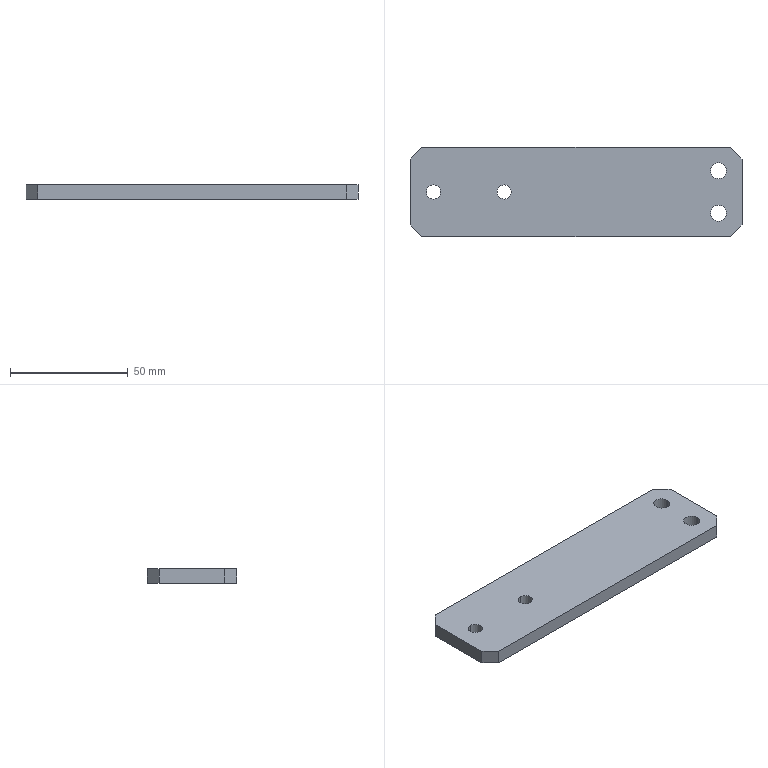Part | STEP file | J014-EBZ05-04-06-Part-1 | 1 solid | 18 faces | box 141 x 38 x 6 mm | volume 31073 mm3 | plane 10 | cylinder 8 | commonest cylinder face diameters 6 x4 6.8 x4
STEP:
#1=CARTESIAN_POINT('',(40.,16.,6.));
#2=VERTEX_POINT('',#1);
#3=CARTESIAN_POINT('',(40.,22.,6.));
#4=VERTEX_POINT('',#3);
#5=CARTESIAN_POINT('',(40.,19.,6.));
#6=DIRECTION('',(0.,0.,-1.));
#7=DIRECTION('',(0.,1.,0.));
#8=AXIS2_PLACEMENT_3D('',#5,#6,#7);
#9=CIRCLE('',#8,3.);
#10=EDGE_CURVE('',#2,#4,#9,.T.);
#11=ORIENTED_EDGE('',*,*,#10,.F.);
#12=CARTESIAN_POINT('',(40.,16.,0.));
#13=VERTEX_POINT('',#12);
#14=CARTESIAN_POINT('',(40.,16.,6.));
#15=DIRECTION('',(0.,0.,-1.));
#16=VECTOR('',#15,1000.);
#17=LINE('',#14,#16);
#18=EDGE_CURVE('',#2,#13,#17,.T.);
#19=ORIENTED_EDGE('',*,*,#18,.T.);
#20=CARTESIAN_POINT('',(40.,22.,0.));
#21=VERTEX_POINT('',#20);
#22=CARTESIAN_POINT('',(40.,19.,0.));
#23=DIRECTION('',(0.,0.,1.));
#24=DIRECTION('',(0.,-1.,0.));
#25=AXIS2_PLACEMENT_3D('',#22,#23,#24);
#26=CIRCLE('',#25,3.);
#27=EDGE_CURVE('',#21,#13,#26,.T.);
#28=ORIENTED_EDGE('',*,*,#27,.F.);
#29=CARTESIAN_POINT('',(40.,22.,6.));
#30=DIRECTION('',(0.,0.,-1.));
#31=VECTOR('',#30,1000.);
#32=LINE('',#29,#31);
#33=EDGE_CURVE('',#4,#21,#32,.T.);
#34=ORIENTED_EDGE('',*,*,#33,.F.);
#35=EDGE_LOOP('',(#11,#19,#28,#34));
#36=FACE_OUTER_BOUND('',#35,.T.);
#37=CARTESIAN_POINT('',(40.,19.,6.));
#38=DIRECTION('',(0.,0.,-1.));
#39=DIRECTION('',(0.,1.,0.));
#40=AXIS2_PLACEMENT_3D('',#37,#38,#39);
#41=CYLINDRICAL_SURFACE('',#40,3.);
#42=ADVANCED_FACE('',(#36),#41,.F.);
#43=CARTESIAN_POINT('',(10.,16.,6.));
#44=VERTEX_POINT('',#43);
#45=CARTESIAN_POINT('',(10.,22.,6.));
#46=VERTEX_POINT('',#45);
#47=CARTESIAN_POINT('',(10.,19.,6.));
#48=DIRECTION('',(0.,0.,-1.));
#49=DIRECTION('',(0.,1.,0.));
#50=AXIS2_PLACEMENT_3D('',#47,#48,#49);
#51=CIRCLE('',#50,3.);
#52=EDGE_CURVE('',#44,#46,#51,.T.);
#53=ORIENTED_EDGE('',*,*,#52,.F.);
#54=CARTESIAN_POINT('',(10.,16.,0.));
#55=VERTEX_POINT('',#54);
#56=CARTESIAN_POINT('',(10.,16.,6.));
#57=DIRECTION('',(0.,0.,-1.));
#58=VECTOR('',#57,1000.);
#59=LINE('',#56,#58);
#60=EDGE_CURVE('',#44,#55,#59,.T.);
#61=ORIENTED_EDGE('',*,*,#60,.T.);
#62=CARTESIAN_POINT('',(10.,22.,0.));
#63=VERTEX_POINT('',#62);
#64=CARTESIAN_POINT('',(10.,19.,0.));
#65=DIRECTION('',(0.,0.,1.));
#66=DIRECTION('',(0.,-1.,0.));
#67=AXIS2_PLACEMENT_3D('',#64,#65,#66);
#68=CIRCLE('',#67,3.);
#69=EDGE_CURVE('',#63,#55,#68,.T.);
#70=ORIENTED_EDGE('',*,*,#69,.F.);
#71=CARTESIAN_POINT('',(10.,22.,6.));
#72=DIRECTION('',(0.,0.,-1.));
#73=VECTOR('',#72,1000.);
#74=LINE('',#71,#73);
#75=EDGE_CURVE('',#46,#63,#74,.T.);
#76=ORIENTED_EDGE('',*,*,#75,.F.);
#77=EDGE_LOOP('',(#53,#61,#70,#76));
#78=FACE_OUTER_BOUND('',#77,.T.);
#79=CARTESIAN_POINT('',(10.,19.,6.));
#80=DIRECTION('',(0.,0.,-1.));
#81=DIRECTION('',(0.,1.,0.));
#82=AXIS2_PLACEMENT_3D('',#79,#80,#81);
#83=CYLINDRICAL_SURFACE('',#82,3.);
#84=ADVANCED_FACE('',(#78),#83,.F.);
#85=CARTESIAN_POINT('',(127.6,10.,0.));
#86=VERTEX_POINT('',#85);
#87=CARTESIAN_POINT('',(134.4,10.,0.));
#88=VERTEX_POINT('',#87);
#89=CARTESIAN_POINT('',(131.,10.,0.));
#90=DIRECTION('',(0.,0.,1.));
#91=DIRECTION('',(1.,0.,0.));
#92=AXIS2_PLACEMENT_3D('',#89,#90,#91);
#93=CIRCLE('',#92,3.4);
#94=EDGE_CURVE('',#86,#88,#93,.T.);
#95=ORIENTED_EDGE('',*,*,#94,.F.);
#96=CARTESIAN_POINT('',(127.6,10.,6.));
#97=VERTEX_POINT('',#96);
#98=CARTESIAN_POINT('',(127.6,10.,0.));
#99=DIRECTION('',(0.,0.,1.));
#100=VECTOR('',#99,1000.);
#101=LINE('',#98,#100);
#102=EDGE_CURVE('',#86,#97,#101,.T.);
#103=ORIENTED_EDGE('',*,*,#102,.T.);
#104=CARTESIAN_POINT('',(134.4,10.,6.));
#105=VERTEX_POINT('',#104);
#106=CARTESIAN_POINT('',(131.,10.,6.));
#107=DIRECTION('',(0.,0.,-1.));
#108=DIRECTION('',(-1.,0.,0.));
#109=AXIS2_PLACEMENT_3D('',#106,#107,#108);
#110=CIRCLE('',#109,3.4);
#111=EDGE_CURVE('',#105,#97,#110,.T.);
#112=ORIENTED_EDGE('',*,*,#111,.F.);
#113=CARTESIAN_POINT('',(134.4,10.,0.));
#114=DIRECTION('',(0.,0.,1.));
#115=VECTOR('',#114,1000.);
#116=LINE('',#113,#115);
#117=EDGE_CURVE('',#88,#105,#116,.T.);
#118=ORIENTED_EDGE('',*,*,#117,.F.);
#119=EDGE_LOOP('',(#95,#103,#112,#118));
#120=FACE_OUTER_BOUND('',#119,.T.);
#121=CARTESIAN_POINT('',(131.,10.,0.));
#122=DIRECTION('',(0.,0.,1.));
#123=DIRECTION('',(1.,0.,0.));
#124=AXIS2_PLACEMENT_3D('',#121,#122,#123);
#125=CYLINDRICAL_SURFACE('',#124,3.4);
#126=ADVANCED_FACE('',(#120),#125,.F.);
#127=CARTESIAN_POINT('',(127.6,28.,0.));
#128=VERTEX_POINT('',#127);
#129=CARTESIAN_POINT('',(134.4,28.,0.));
#130=VERTEX_POINT('',#129);
#131=CARTESIAN_POINT('',(131.,28.,0.));
#132=DIRECTION('',(0.,0.,1.));
#133=DIRECTION('',(1.,0.,0.));
#134=AXIS2_PLACEMENT_3D('',#131,#132,#133);
#135=CIRCLE('',#134,3.4);
#136=EDGE_CURVE('',#128,#130,#135,.T.);
#137=ORIENTED_EDGE('',*,*,#136,.F.);
#138=CARTESIAN_POINT('',(127.6,28.,6.));
#139=VERTEX_POINT('',#138);
#140=CARTESIAN_POINT('',(127.6,28.,0.));
#141=DIRECTION('',(0.,0.,1.));
#142=VECTOR('',#141,1000.);
#143=LINE('',#140,#142);
#144=EDGE_CURVE('',#128,#139,#143,.T.);
#145=ORIENTED_EDGE('',*,*,#144,.T.);
#146=CARTESIAN_POINT('',(134.4,28.,6.));
#147=VERTEX_POINT('',#146);
#148=CARTESIAN_POINT('',(131.,28.,6.));
#149=DIRECTION('',(0.,0.,-1.));
#150=DIRECTION('',(-1.,0.,0.));
#151=AXIS2_PLACEMENT_3D('',#148,#149,#150);
#152=CIRCLE('',#151,3.4);
#153=EDGE_CURVE('',#147,#139,#152,.T.);
#154=ORIENTED_EDGE('',*,*,#153,.F.);
#155=CARTESIAN_POINT('',(134.4,28.,0.));
#156=DIRECTION('',(0.,0.,1.));
#157=VECTOR('',#156,1000.);
#158=LINE('',#155,#157);
#159=EDGE_CURVE('',#130,#147,#158,.T.);
#160=ORIENTED_EDGE('',*,*,#159,.F.);
#161=EDGE_LOOP('',(#137,#145,#154,#160));
#162=FACE_OUTER_BOUND('',#161,.T.);
#163=CARTESIAN_POINT('',(131.,28.,0.));
#164=DIRECTION('',(0.,0.,1.));
#165=DIRECTION('',(1.,0.,0.));
#166=AXIS2_PLACEMENT_3D('',#163,#164,#165);
#167=CYLINDRICAL_SURFACE('',#166,3.4);
#168=ADVANCED_FACE('',(#162),#167,.F.);
#169=ORIENTED_EDGE('',*,*,#27,.T.);
#170=CARTESIAN_POINT('',(40.,19.,0.));
#171=DIRECTION('',(0.,0.,1.));
#172=DIRECTION('',(0.,-1.,0.));
#173=AXIS2_PLACEMENT_3D('',#170,#171,#172);
#174=CIRCLE('',#173,3.);
#175=EDGE_CURVE('',#13,#21,#174,.T.);
#176=ORIENTED_EDGE('',*,*,#175,.T.);
#177=EDGE_LOOP('',(#169,#176));
#178=FACE_BOUND('',#177,.T.);
#179=ORIENTED_EDGE('',*,*,#69,.T.);
#180=CARTESIAN_POINT('',(10.,19.,0.));
#181=DIRECTION('',(0.,0.,1.));
#182=DIRECTION('',(0.,-1.,0.));
#183=AXIS2_PLACEMENT_3D('',#180,#181,#182);
#184=CIRCLE('',#183,3.);
#185=EDGE_CURVE('',#55,#63,#184,.T.);
#186=ORIENTED_EDGE('',*,*,#185,.T.);
#187=EDGE_LOOP('',(#179,#186));
#188=FACE_BOUND('',#187,.T.);
#189=CARTESIAN_POINT('',(131.,10.,0.));
#190=DIRECTION('',(0.,0.,1.));
#191=DIRECTION('',(1.,0.,0.));
#192=AXIS2_PLACEMENT_3D('',#189,#190,#191);
#193=CIRCLE('',#192,3.4);
#194=EDGE_CURVE('',#88,#86,#193,.T.);
#195=ORIENTED_EDGE('',*,*,#194,.T.);
#196=ORIENTED_EDGE('',*,*,#94,.T.);
#197=EDGE_LOOP('',(#195,#196));
#198=FACE_BOUND('',#197,.T.);
#199=CARTESIAN_POINT('',(131.,28.,0.));
#200=DIRECTION('',(0.,0.,1.));
#201=DIRECTION('',(1.,0.,0.));
#202=AXIS2_PLACEMENT_3D('',#199,#200,#201);
#203=CIRCLE('',#202,3.4);
#204=EDGE_CURVE('',#130,#128,#203,.T.);
#205=ORIENTED_EDGE('',*,*,#204,.T.);
#206=ORIENTED_EDGE('',*,*,#136,.T.);
#207=EDGE_LOOP('',(#205,#206));
#208=FACE_BOUND('',#207,.T.);
#209=CARTESIAN_POINT('',(136.,38.,0.));
#210=VERTEX_POINT('',#209);
#211=CARTESIAN_POINT('',(5.,38.,0.));
#212=VERTEX_POINT('',#211);
#213=CARTESIAN_POINT('',(70.5,38.,0.));
#214=DIRECTION('',(-1.,0.,0.));
#215=VECTOR('',#214,1000.);
#216=LINE('',#213,#215);
#217=EDGE_CURVE('',#210,#212,#216,.T.);
#218=ORIENTED_EDGE('',*,*,#217,.F.);
#219=CARTESIAN_POINT('',(141.,33.,0.));
#220=VERTEX_POINT('',#219);
#221=CARTESIAN_POINT('',(112.75,61.25,0.));
#222=DIRECTION('',(0.7071,-0.7071,0.));
#223=VECTOR('',#222,1000.);
#224=LINE('',#221,#223);
#225=EDGE_CURVE('',#210,#220,#224,.T.);
#226=ORIENTED_EDGE('',*,*,#225,.T.);
#227=CARTESIAN_POINT('',(141.,5.,0.));
#228=VERTEX_POINT('',#227);
#229=CARTESIAN_POINT('',(141.,19.,0.));
#230=DIRECTION('',(0.,1.,0.));
#231=VECTOR('',#230,1000.);
#232=LINE('',#229,#231);
#233=EDGE_CURVE('',#228,#220,#232,.T.);
#234=ORIENTED_EDGE('',*,*,#233,.F.);
#235=CARTESIAN_POINT('',(136.,0.,0.));
#236=VERTEX_POINT('',#235);
#237=CARTESIAN_POINT('',(112.75,-23.25,0.));
#238=DIRECTION('',(-0.7071,-0.7071,0.));
#239=VECTOR('',#238,1000.);
#240=LINE('',#237,#239);
#241=EDGE_CURVE('',#228,#236,#240,.T.);
#242=ORIENTED_EDGE('',*,*,#241,.T.);
#243=CARTESIAN_POINT('',(5.,0.,0.));
#244=VERTEX_POINT('',#243);
#245=CARTESIAN_POINT('',(70.5,0.,0.));
#246=DIRECTION('',(1.,0.,0.));
#247=VECTOR('',#246,1000.);
#248=LINE('',#245,#247);
#249=EDGE_CURVE('',#244,#236,#248,.T.);
#250=ORIENTED_EDGE('',*,*,#249,.F.);
#251=CARTESIAN_POINT('',(0.,5.,0.));
#252=VERTEX_POINT('',#251);
#253=CARTESIAN_POINT('',(28.25,-23.25,0.));
#254=DIRECTION('',(-0.7071,0.7071,0.));
#255=VECTOR('',#254,1000.);
#256=LINE('',#253,#255);
#257=EDGE_CURVE('',#244,#252,#256,.T.);
#258=ORIENTED_EDGE('',*,*,#257,.T.);
#259=CARTESIAN_POINT('',(0.,33.,0.));
#260=VERTEX_POINT('',#259);
#261=CARTESIAN_POINT('',(0.,19.,0.));
#262=DIRECTION('',(0.,-1.,0.));
#263=VECTOR('',#262,1000.);
#264=LINE('',#261,#263);
#265=EDGE_CURVE('',#260,#252,#264,.T.);
#266=ORIENTED_EDGE('',*,*,#265,.F.);
#267=CARTESIAN_POINT('',(28.25,61.25,0.));
#268=DIRECTION('',(0.7071,0.7071,0.));
#269=VECTOR('',#268,1000.);
#270=LINE('',#267,#269);
#271=EDGE_CURVE('',#260,#212,#270,.T.);
#272=ORIENTED_EDGE('',*,*,#271,.T.);
#273=EDGE_LOOP('',(#218,#226,#234,#242,#250,#258,#266,#272));
#274=FACE_OUTER_BOUND('',#273,.T.);
#275=CARTESIAN_POINT('',(70.5,19.,0.));
#276=DIRECTION('',(0.,0.,-1.));
#277=DIRECTION('',(0.,1.,0.));
#278=AXIS2_PLACEMENT_3D('',#275,#276,#277);
#279=PLANE('',#278);
#280=ADVANCED_FACE('',(#178,#188,#198,#208,#274),#279,.T.);
#281=ORIENTED_EDGE('',*,*,#265,.T.);
#282=CARTESIAN_POINT('',(0.,5.,6.));
#283=VERTEX_POINT('',#282);
#284=CARTESIAN_POINT('',(0.,5.,6.));
#285=DIRECTION('',(0.,0.,1.));
#286=VECTOR('',#285,1000.);
#287=LINE('',#284,#286);
#288=EDGE_CURVE('',#252,#283,#287,.T.);
#289=ORIENTED_EDGE('',*,*,#288,.T.);
#290=CARTESIAN_POINT('',(0.,33.,6.));
#291=VERTEX_POINT('',#290);
#292=CARTESIAN_POINT('',(0.,19.,6.));
#293=DIRECTION('',(0.,1.,0.));
#294=VECTOR('',#293,1000.);
#295=LINE('',#292,#294);
#296=EDGE_CURVE('',#283,#291,#295,.T.);
#297=ORIENTED_EDGE('',*,*,#296,.T.);
#298=CARTESIAN_POINT('',(0.,33.,6.));
#299=DIRECTION('',(0.,0.,-1.));
#300=VECTOR('',#299,1000.);
#301=LINE('',#298,#300);
#302=EDGE_CURVE('',#291,#260,#301,.T.);
#303=ORIENTED_EDGE('',*,*,#302,.T.);
#304=EDGE_LOOP('',(#281,#289,#297,#303));
#305=FACE_OUTER_BOUND('',#304,.T.);
#306=CARTESIAN_POINT('',(0.,19.,6.));
#307=DIRECTION('',(-1.,0.,0.));
#308=DIRECTION('',(0.,0.,1.));
#309=AXIS2_PLACEMENT_3D('',#306,#307,#308);
#310=PLANE('',#309);
#311=ADVANCED_FACE('',(#305),#310,.T.);
#312=ORIENTED_EDGE('',*,*,#249,.T.);
#313=CARTESIAN_POINT('',(136.,0.,6.));
#314=VERTEX_POINT('',#313);
#315=CARTESIAN_POINT('',(136.,0.,6.));
#316=DIRECTION('',(0.,0.,1.));
#317=VECTOR('',#316,1000.);
#318=LINE('',#315,#317);
#319=EDGE_CURVE('',#236,#314,#318,.T.);
#320=ORIENTED_EDGE('',*,*,#319,.T.);
#321=CARTESIAN_POINT('',(5.,0.,6.));
#322=VERTEX_POINT('',#321);
#323=CARTESIAN_POINT('',(70.5,0.,6.));
#324=DIRECTION('',(-1.,0.,0.));
#325=VECTOR('',#324,1000.);
#326=LINE('',#323,#325);
#327=EDGE_CURVE('',#314,#322,#326,.T.);
#328=ORIENTED_EDGE('',*,*,#327,.T.);
#329=CARTESIAN_POINT('',(5.,0.,6.));
#330=DIRECTION('',(0.,0.,-1.));
#331=VECTOR('',#330,1000.);
#332=LINE('',#329,#331);
#333=EDGE_CURVE('',#322,#244,#332,.T.);
#334=ORIENTED_EDGE('',*,*,#333,.T.);
#335=EDGE_LOOP('',(#312,#320,#328,#334));
#336=FACE_OUTER_BOUND('',#335,.T.);
#337=CARTESIAN_POINT('',(70.5,0.,6.));
#338=DIRECTION('',(0.,-1.,0.));
#339=DIRECTION('',(0.,0.,-1.));
#340=AXIS2_PLACEMENT_3D('',#337,#338,#339);
#341=PLANE('',#340);
#342=ADVANCED_FACE('',(#336),#341,.T.);
#343=ORIENTED_EDGE('',*,*,#233,.T.);
#344=CARTESIAN_POINT('',(141.,33.,6.));
#345=VERTEX_POINT('',#344);
#346=CARTESIAN_POINT('',(141.,33.,6.));
#347=DIRECTION('',(0.,0.,1.));
#348=VECTOR('',#347,1000.);
#349=LINE('',#346,#348);
#350=EDGE_CURVE('',#220,#345,#349,.T.);
#351=ORIENTED_EDGE('',*,*,#350,.T.);
#352=CARTESIAN_POINT('',(141.,5.,6.));
#353=VERTEX_POINT('',#352);
#354=CARTESIAN_POINT('',(141.,19.,6.));
#355=DIRECTION('',(0.,-1.,0.));
#356=VECTOR('',#355,1000.);
#357=LINE('',#354,#356);
#358=EDGE_CURVE('',#345,#353,#357,.T.);
#359=ORIENTED_EDGE('',*,*,#358,.T.);
#360=CARTESIAN_POINT('',(141.,5.,6.));
#361=DIRECTION('',(0.,0.,-1.));
#362=VECTOR('',#361,1000.);
#363=LINE('',#360,#362);
#364=EDGE_CURVE('',#353,#228,#363,.T.);
#365=ORIENTED_EDGE('',*,*,#364,.T.);
#366=EDGE_LOOP('',(#343,#351,#359,#365));
#367=FACE_OUTER_BOUND('',#366,.T.);
#368=CARTESIAN_POINT('',(141.,19.,6.));
#369=DIRECTION('',(1.,0.,0.));
#370=DIRECTION('',(0.,0.,-1.));
#371=AXIS2_PLACEMENT_3D('',#368,#369,#370);
#372=PLANE('',#371);
#373=ADVANCED_FACE('',(#367),#372,.T.);
#374=CARTESIAN_POINT('',(40.,19.,6.));
#375=DIRECTION('',(0.,0.,-1.));
#376=DIRECTION('',(0.,1.,0.));
#377=AXIS2_PLACEMENT_3D('',#374,#375,#376);
#378=CIRCLE('',#377,3.);
#379=EDGE_CURVE('',#4,#2,#378,.T.);
#380=ORIENTED_EDGE('',*,*,#379,.T.);
#381=ORIENTED_EDGE('',*,*,#10,.T.);
#382=EDGE_LOOP('',(#380,#381));
#383=FACE_BOUND('',#382,.T.);
#384=CARTESIAN_POINT('',(10.,19.,6.));
#385=DIRECTION('',(0.,0.,-1.));
#386=DIRECTION('',(0.,1.,0.));
#387=AXIS2_PLACEMENT_3D('',#384,#385,#386);
#388=CIRCLE('',#387,3.);
#389=EDGE_CURVE('',#46,#44,#388,.T.);
#390=ORIENTED_EDGE('',*,*,#389,.T.);
#391=ORIENTED_EDGE('',*,*,#52,.T.);
#392=EDGE_LOOP('',(#390,#391));
#393=FACE_BOUND('',#392,.T.);
#394=ORIENTED_EDGE('',*,*,#111,.T.);
#395=CARTESIAN_POINT('',(131.,10.,6.));
#396=DIRECTION('',(0.,0.,-1.));
#397=DIRECTION('',(-1.,0.,0.));
#398=AXIS2_PLACEMENT_3D('',#395,#396,#397);
#399=CIRCLE('',#398,3.4);
#400=EDGE_CURVE('',#97,#105,#399,.T.);
#401=ORIENTED_EDGE('',*,*,#400,.T.);
#402=EDGE_LOOP('',(#394,#401));
#403=FACE_BOUND('',#402,.T.);
#404=ORIENTED_EDGE('',*,*,#153,.T.);
#405=CARTESIAN_POINT('',(131.,28.,6.));
#406=DIRECTION('',(0.,0.,-1.));
#407=DIRECTION('',(-1.,0.,0.));
#408=AXIS2_PLACEMENT_3D('',#405,#406,#407);
#409=CIRCLE('',#408,3.4);
#410=EDGE_CURVE('',#139,#147,#409,.T.);
#411=ORIENTED_EDGE('',*,*,#410,.T.);
#412=EDGE_LOOP('',(#404,#411));
#413=FACE_BOUND('',#412,.T.);
#414=ORIENTED_EDGE('',*,*,#358,.F.);
#415=CARTESIAN_POINT('',(136.,38.,6.));
#416=VERTEX_POINT('',#415);
#417=CARTESIAN_POINT('',(112.75,61.25,6.));
#418=DIRECTION('',(-0.7071,0.7071,0.));
#419=VECTOR('',#418,1000.);
#420=LINE('',#417,#419);
#421=EDGE_CURVE('',#345,#416,#420,.T.);
#422=ORIENTED_EDGE('',*,*,#421,.T.);
#423=CARTESIAN_POINT('',(5.,38.,6.));
#424=VERTEX_POINT('',#423);
#425=CARTESIAN_POINT('',(70.5,38.,6.));
#426=DIRECTION('',(1.,0.,0.));
#427=VECTOR('',#426,1000.);
#428=LINE('',#425,#427);
#429=EDGE_CURVE('',#424,#416,#428,.T.);
#430=ORIENTED_EDGE('',*,*,#429,.F.);
#431=CARTESIAN_POINT('',(28.25,61.25,6.));
#432=DIRECTION('',(-0.7071,-0.7071,0.));
#433=VECTOR('',#432,1000.);
#434=LINE('',#431,#433);
#435=EDGE_CURVE('',#424,#291,#434,.T.);
#436=ORIENTED_EDGE('',*,*,#435,.T.);
#437=ORIENTED_EDGE('',*,*,#296,.F.);
#438=CARTESIAN_POINT('',(28.25,-23.25,6.));
#439=DIRECTION('',(0.7071,-0.7071,0.));
#440=VECTOR('',#439,1000.);
#441=LINE('',#438,#440);
#442=EDGE_CURVE('',#283,#322,#441,.T.);
#443=ORIENTED_EDGE('',*,*,#442,.T.);
#444=ORIENTED_EDGE('',*,*,#327,.F.);
#445=CARTESIAN_POINT('',(112.75,-23.25,6.));
#446=DIRECTION('',(0.7071,0.7071,0.));
#447=VECTOR('',#446,1000.);
#448=LINE('',#445,#447);
#449=EDGE_CURVE('',#314,#353,#448,.T.);
#450=ORIENTED_EDGE('',*,*,#449,.T.);
#451=EDGE_LOOP('',(#414,#422,#430,#436,#437,#443,#444,#450));
#452=FACE_OUTER_BOUND('',#451,.T.);
#453=CARTESIAN_POINT('',(70.5,19.,6.));
#454=DIRECTION('',(0.,0.,1.));
#455=DIRECTION('',(0.,-1.,0.));
#456=AXIS2_PLACEMENT_3D('',#453,#454,#455);
#457=PLANE('',#456);
#458=ADVANCED_FACE('',(#383,#393,#403,#413,#452),#457,.T.);
#459=ORIENTED_EDGE('',*,*,#429,.T.);
#460=CARTESIAN_POINT('',(136.,38.,6.));
#461=DIRECTION('',(0.,0.,-1.));
#462=VECTOR('',#461,1000.);
#463=LINE('',#460,#462);
#464=EDGE_CURVE('',#416,#210,#463,.T.);
#465=ORIENTED_EDGE('',*,*,#464,.T.);
#466=ORIENTED_EDGE('',*,*,#217,.T.);
#467=CARTESIAN_POINT('',(5.,38.,6.));
#468=DIRECTION('',(0.,0.,1.));
#469=VECTOR('',#468,1000.);
#470=LINE('',#467,#469);
#471=EDGE_CURVE('',#212,#424,#470,.T.);
#472=ORIENTED_EDGE('',*,*,#471,.T.);
#473=EDGE_LOOP('',(#459,#465,#466,#472));
#474=FACE_OUTER_BOUND('',#473,.T.);
#475=CARTESIAN_POINT('',(70.5,38.,6.));
#476=DIRECTION('',(0.,1.,0.));
#477=DIRECTION('',(0.,0.,1.));
#478=AXIS2_PLACEMENT_3D('',#475,#476,#477);
#479=PLANE('',#478);
#480=ADVANCED_FACE('',(#474),#479,.T.);
#481=ORIENTED_EDGE('',*,*,#144,.F.);
#482=ORIENTED_EDGE('',*,*,#204,.F.);
#483=ORIENTED_EDGE('',*,*,#159,.T.);
#484=ORIENTED_EDGE('',*,*,#410,.F.);
#485=EDGE_LOOP('',(#481,#482,#483,#484));
#486=FACE_OUTER_BOUND('',#485,.T.);
#487=CARTESIAN_POINT('',(131.,28.,0.));
#488=DIRECTION('',(0.,0.,1.));
#489=DIRECTION('',(1.,0.,0.));
#490=AXIS2_PLACEMENT_3D('',#487,#488,#489);
#491=CYLINDRICAL_SURFACE('',#490,3.4);
#492=ADVANCED_FACE('',(#486),#491,.F.);
#493=ORIENTED_EDGE('',*,*,#102,.F.);
#494=ORIENTED_EDGE('',*,*,#194,.F.);
#495=ORIENTED_EDGE('',*,*,#117,.T.);
#496=ORIENTED_EDGE('',*,*,#400,.F.);
#497=EDGE_LOOP('',(#493,#494,#495,#496));
#498=FACE_OUTER_BOUND('',#497,.T.);
#499=CARTESIAN_POINT('',(131.,10.,0.));
#500=DIRECTION('',(0.,0.,1.));
#501=DIRECTION('',(1.,0.,0.));
#502=AXIS2_PLACEMENT_3D('',#499,#500,#501);
#503=CYLINDRICAL_SURFACE('',#502,3.4);
#504=ADVANCED_FACE('',(#498),#503,.F.);
#505=ORIENTED_EDGE('',*,*,#60,.F.);
#506=ORIENTED_EDGE('',*,*,#389,.F.);
#507=ORIENTED_EDGE('',*,*,#75,.T.);
#508=ORIENTED_EDGE('',*,*,#185,.F.);
#509=EDGE_LOOP('',(#505,#506,#507,#508));
#510=FACE_OUTER_BOUND('',#509,.T.);
#511=CARTESIAN_POINT('',(10.,19.,6.));
#512=DIRECTION('',(0.,0.,-1.));
#513=DIRECTION('',(0.,1.,0.));
#514=AXIS2_PLACEMENT_3D('',#511,#512,#513);
#515=CYLINDRICAL_SURFACE('',#514,3.);
#516=ADVANCED_FACE('',(#510),#515,.F.);
#517=ORIENTED_EDGE('',*,*,#18,.F.);
#518=ORIENTED_EDGE('',*,*,#379,.F.);
#519=ORIENTED_EDGE('',*,*,#33,.T.);
#520=ORIENTED_EDGE('',*,*,#175,.F.);
#521=EDGE_LOOP('',(#517,#518,#519,#520));
#522=FACE_OUTER_BOUND('',#521,.T.);
#523=CARTESIAN_POINT('',(40.,19.,6.));
#524=DIRECTION('',(0.,0.,-1.));
#525=DIRECTION('',(0.,1.,0.));
#526=AXIS2_PLACEMENT_3D('',#523,#524,#525);
#527=CYLINDRICAL_SURFACE('',#526,3.);
#528=ADVANCED_FACE('',(#522),#527,.F.);
#529=ORIENTED_EDGE('',*,*,#435,.F.);
#530=ORIENTED_EDGE('',*,*,#471,.F.);
#531=ORIENTED_EDGE('',*,*,#271,.F.);
#532=ORIENTED_EDGE('',*,*,#302,.F.);
#533=EDGE_LOOP('',(#529,#530,#531,#532));
#534=FACE_OUTER_BOUND('',#533,.T.);
#535=CARTESIAN_POINT('',(0.,33.,6.));
#536=DIRECTION('',(0.7071,-0.7071,0.));
#537=DIRECTION('',(0.,0.,-1.));
#538=AXIS2_PLACEMENT_3D('',#535,#536,#537);
#539=PLANE('',#538);
#540=ADVANCED_FACE('',(#534),#539,.F.);
#541=ORIENTED_EDGE('',*,*,#442,.F.);
#542=ORIENTED_EDGE('',*,*,#288,.F.);
#543=ORIENTED_EDGE('',*,*,#257,.F.);
#544=ORIENTED_EDGE('',*,*,#333,.F.);
#545=EDGE_LOOP('',(#541,#542,#543,#544));
#546=FACE_OUTER_BOUND('',#545,.T.);
#547=CARTESIAN_POINT('',(5.,0.,6.));
#548=DIRECTION('',(0.7071,0.7071,0.));
#549=DIRECTION('',(0.,0.,-1.));
#550=AXIS2_PLACEMENT_3D('',#547,#548,#549);
#551=PLANE('',#550);
#552=ADVANCED_FACE('',(#546),#551,.F.);
#553=ORIENTED_EDGE('',*,*,#449,.F.);
#554=ORIENTED_EDGE('',*,*,#319,.F.);
#555=ORIENTED_EDGE('',*,*,#241,.F.);
#556=ORIENTED_EDGE('',*,*,#364,.F.);
#557=EDGE_LOOP('',(#553,#554,#555,#556));
#558=FACE_OUTER_BOUND('',#557,.T.);
#559=CARTESIAN_POINT('',(141.,5.,6.));
#560=DIRECTION('',(-0.7071,0.7071,0.));
#561=DIRECTION('',(0.,0.,-1.));
#562=AXIS2_PLACEMENT_3D('',#559,#560,#561);
#563=PLANE('',#562);
#564=ADVANCED_FACE('',(#558),#563,.F.);
#565=ORIENTED_EDGE('',*,*,#421,.F.);
#566=ORIENTED_EDGE('',*,*,#350,.F.);
#567=ORIENTED_EDGE('',*,*,#225,.F.);
#568=ORIENTED_EDGE('',*,*,#464,.F.);
#569=EDGE_LOOP('',(#565,#566,#567,#568));
#570=FACE_OUTER_BOUND('',#569,.T.);
#571=CARTESIAN_POINT('',(136.,38.,6.));
#572=DIRECTION('',(-0.7071,-0.7071,0.));
#573=DIRECTION('',(0.,0.,-1.));
#574=AXIS2_PLACEMENT_3D('',#571,#572,#573);
#575=PLANE('',#574);
#576=ADVANCED_FACE('',(#570),#575,.F.);
#577=CLOSED_SHELL('',(#42,#84,#126,#168,#280,#311,#342,#373,#458,#480,#492,#504,#516,#528,#540,#552,#564,#576));
#578=MANIFOLD_SOLID_BREP('',#577);
#579=CARTESIAN_POINT('',(0.,0.,0.));
#580=DIRECTION('',(0.,0.,1.));
#581=DIRECTION('',(1.,0.,0.));
#582=AXIS2_PLACEMENT_3D('',#579,#580,#581);
#583=(LENGTH_UNIT()NAMED_UNIT(*)SI_UNIT(.MILLI.,.METRE.));
#584=UNCERTAINTY_MEASURE_WITH_UNIT(LENGTH_MEASURE(0.00001),#583,'','');
#585=(NAMED_UNIT(*)PLANE_ANGLE_UNIT()SI_UNIT($,.RADIAN.));
#586=(NAMED_UNIT(*)SI_UNIT($,.STERADIAN.)SOLID_ANGLE_UNIT());
#587=(GEOMETRIC_REPRESENTATION_CONTEXT(3)GLOBAL_UNCERTAINTY_ASSIGNED_CONTEXT((#584))GLOBAL_UNIT_ASSIGNED_CONTEXT((#583,#585,#586))REPRESENTATION_CONTEXT('',''));
#588=ADVANCED_BREP_SHAPE_REPRESENTATION('',(#578,#582),#587);